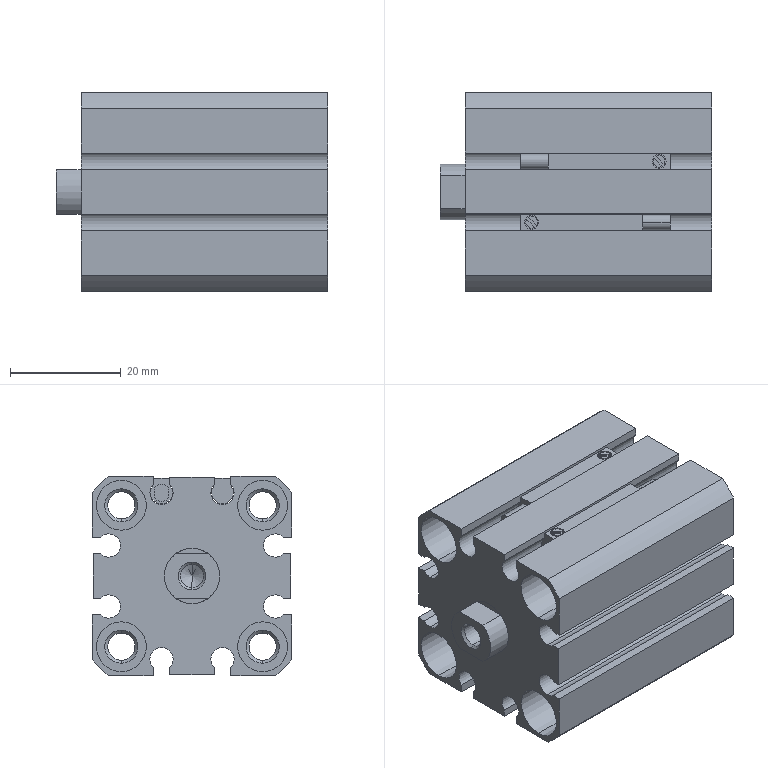Part | STEP file | 4 solids | 212 faces | box 49 x 36 x 36 mm | volume 41848 mm3 | cylinder 95 | plane 73 | cone 44 | commonest cylinder face diameters 4.2 x18 4.917 x16 9 x16 5.4 x8 2.1 x6 2.7 x6